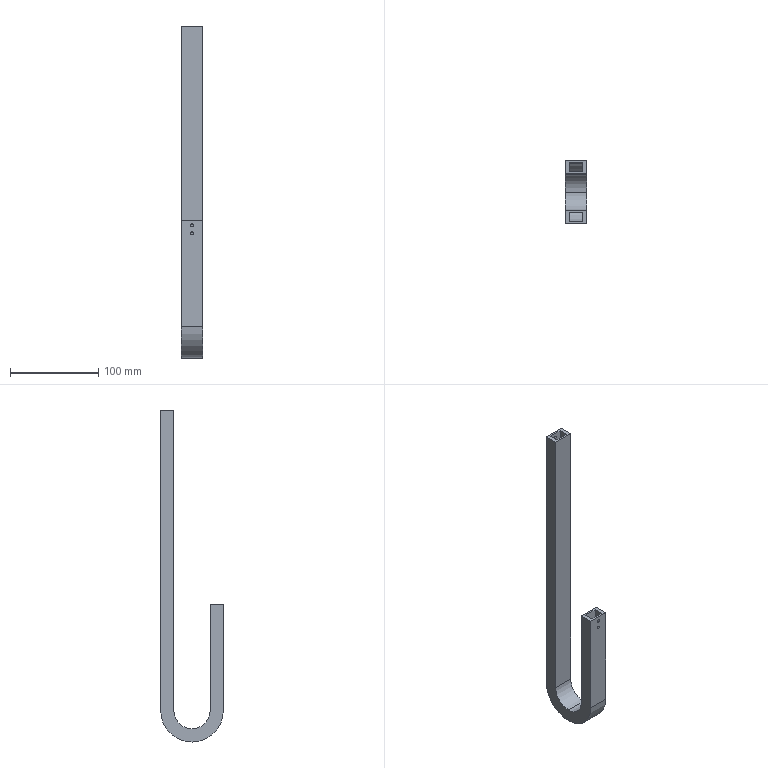Part | SolidWorks | features ICE 2, Sweep 1 | 1 solid | 30 faces | box 24 x 71 x 375.5 mm | volume 114976 mm3 | cylinder 16 | plane 14 | commonest cylinder face diameters 3.5 x8 41 x2 46 x2 66 x2 71 x2
STEP:
#1=CARTESIAN_POINT('',(-1.75,-5.,-14.5));
#2=VERTEX_POINT('',#1);
#3=CARTESIAN_POINT('',(1.75,-5.,-14.5));
#4=VERTEX_POINT('',#3);
#5=CARTESIAN_POINT('',(0.,-5.,-14.5));
#6=DIRECTION('',(0.,-1.,0.));
#7=DIRECTION('',(1.,0.,0.));
#8=AXIS2_PLACEMENT_3D('',#5,#6,#7);
#9=CIRCLE('',#8,1.75);
#10=EDGE_CURVE('',#2,#4,#9,.T.);
#11=ORIENTED_EDGE('',*,*,#10,.F.);
#12=CARTESIAN_POINT('',(-1.75,-7.5,-14.5));
#13=VERTEX_POINT('',#12);
#14=CARTESIAN_POINT('',(-1.75,-2.5,-14.5));
#15=DIRECTION('',(0.,-1.,0.));
#16=VECTOR('',#15,1000.);
#17=LINE('',#14,#16);
#18=EDGE_CURVE('',#2,#13,#17,.T.);
#19=ORIENTED_EDGE('',*,*,#18,.T.);
#20=CARTESIAN_POINT('',(1.75,-7.5,-14.5));
#21=VERTEX_POINT('',#20);
#22=CARTESIAN_POINT('',(0.,-7.5,-14.5));
#23=DIRECTION('',(0.,-1.,0.));
#24=DIRECTION('',(1.,0.,0.));
#25=AXIS2_PLACEMENT_3D('',#22,#23,#24);
#26=CIRCLE('',#25,1.75);
#27=EDGE_CURVE('',#13,#21,#26,.T.);
#28=ORIENTED_EDGE('',*,*,#27,.T.);
#29=CARTESIAN_POINT('',(1.75,-2.5,-14.5));
#30=DIRECTION('',(0.,-1.,0.));
#31=VECTOR('',#30,1000.);
#32=LINE('',#29,#31);
#33=EDGE_CURVE('',#4,#21,#32,.T.);
#34=ORIENTED_EDGE('',*,*,#33,.F.);
#35=EDGE_LOOP('',(#11,#19,#28,#34));
#36=FACE_OUTER_BOUND('',#35,.T.);
#37=CARTESIAN_POINT('',(0.,-2.5,-14.5));
#38=DIRECTION('',(0.,-1.,0.));
#39=DIRECTION('',(1.,0.,0.));
#40=AXIS2_PLACEMENT_3D('',#37,#38,#39);
#41=CYLINDRICAL_SURFACE('',#40,1.75);
#42=ADVANCED_FACE('',(#36),#41,.F.);
#43=CARTESIAN_POINT('',(-1.75,-5.,-5.5));
#44=VERTEX_POINT('',#43);
#45=CARTESIAN_POINT('',(1.75,-5.,-5.5));
#46=VERTEX_POINT('',#45);
#47=CARTESIAN_POINT('',(0.,-5.,-5.5));
#48=DIRECTION('',(0.,-1.,0.));
#49=DIRECTION('',(1.,0.,0.));
#50=AXIS2_PLACEMENT_3D('',#47,#48,#49);
#51=CIRCLE('',#50,1.75);
#52=EDGE_CURVE('',#44,#46,#51,.T.);
#53=ORIENTED_EDGE('',*,*,#52,.F.);
#54=CARTESIAN_POINT('',(-1.75,-7.5,-5.5));
#55=VERTEX_POINT('',#54);
#56=CARTESIAN_POINT('',(-1.75,-2.5,-5.5));
#57=DIRECTION('',(0.,-1.,0.));
#58=VECTOR('',#57,1000.);
#59=LINE('',#56,#58);
#60=EDGE_CURVE('',#44,#55,#59,.T.);
#61=ORIENTED_EDGE('',*,*,#60,.T.);
#62=CARTESIAN_POINT('',(1.75,-7.5,-5.5));
#63=VERTEX_POINT('',#62);
#64=CARTESIAN_POINT('',(0.,-7.5,-5.5));
#65=DIRECTION('',(0.,-1.,0.));
#66=DIRECTION('',(1.,0.,0.));
#67=AXIS2_PLACEMENT_3D('',#64,#65,#66);
#68=CIRCLE('',#67,1.75);
#69=EDGE_CURVE('',#55,#63,#68,.T.);
#70=ORIENTED_EDGE('',*,*,#69,.T.);
#71=CARTESIAN_POINT('',(1.75,-2.5,-5.5));
#72=DIRECTION('',(0.,-1.,0.));
#73=VECTOR('',#72,1000.);
#74=LINE('',#71,#73);
#75=EDGE_CURVE('',#46,#63,#74,.T.);
#76=ORIENTED_EDGE('',*,*,#75,.F.);
#77=EDGE_LOOP('',(#53,#61,#70,#76));
#78=FACE_OUTER_BOUND('',#77,.T.);
#79=CARTESIAN_POINT('',(0.,-2.5,-5.5));
#80=DIRECTION('',(0.,-1.,0.));
#81=DIRECTION('',(1.,0.,0.));
#82=AXIS2_PLACEMENT_3D('',#79,#80,#81);
#83=CYLINDRICAL_SURFACE('',#82,1.75);
#84=ADVANCED_FACE('',(#78),#83,.F.);
#85=CARTESIAN_POINT('',(-1.75,61.,205.5));
#86=VERTEX_POINT('',#85);
#87=CARTESIAN_POINT('',(1.75,61.,205.5));
#88=VERTEX_POINT('',#87);
#89=CARTESIAN_POINT('',(0.,61.,205.5));
#90=DIRECTION('',(0.,-1.,0.));
#91=DIRECTION('',(0.,0.,-1.));
#92=AXIS2_PLACEMENT_3D('',#89,#90,#91);
#93=CIRCLE('',#92,1.75);
#94=EDGE_CURVE('',#86,#88,#93,.T.);
#95=ORIENTED_EDGE('',*,*,#94,.T.);
#96=CARTESIAN_POINT('',(1.75,63.5,205.5));
#97=VERTEX_POINT('',#96);
#98=CARTESIAN_POINT('',(1.75,58.5,205.5));
#99=DIRECTION('',(0.,1.,0.));
#100=VECTOR('',#99,1000.);
#101=LINE('',#98,#100);
#102=EDGE_CURVE('',#88,#97,#101,.T.);
#103=ORIENTED_EDGE('',*,*,#102,.T.);
#104=CARTESIAN_POINT('',(-1.75,63.5,205.5));
#105=VERTEX_POINT('',#104);
#106=CARTESIAN_POINT('',(0.,63.5,205.5));
#107=DIRECTION('',(0.,1.,0.));
#108=DIRECTION('',(-1.,0.,0.));
#109=AXIS2_PLACEMENT_3D('',#106,#107,#108);
#110=CIRCLE('',#109,1.75);
#111=EDGE_CURVE('',#97,#105,#110,.T.);
#112=ORIENTED_EDGE('',*,*,#111,.T.);
#113=CARTESIAN_POINT('',(-1.75,58.5,205.5));
#114=DIRECTION('',(0.,1.,0.));
#115=VECTOR('',#114,1000.);
#116=LINE('',#113,#115);
#117=EDGE_CURVE('',#86,#105,#116,.T.);
#118=ORIENTED_EDGE('',*,*,#117,.F.);
#119=EDGE_LOOP('',(#95,#103,#112,#118));
#120=FACE_OUTER_BOUND('',#119,.T.);
#121=CARTESIAN_POINT('',(0.,58.5,205.5));
#122=DIRECTION('',(0.,1.,0.));
#123=DIRECTION('',(-1.,0.,0.));
#124=AXIS2_PLACEMENT_3D('',#121,#122,#123);
#125=CYLINDRICAL_SURFACE('',#124,1.75);
#126=ADVANCED_FACE('',(#120),#125,.F.);
#127=CARTESIAN_POINT('',(-1.75,61.,214.5));
#128=VERTEX_POINT('',#127);
#129=CARTESIAN_POINT('',(1.75,61.,214.5));
#130=VERTEX_POINT('',#129);
#131=CARTESIAN_POINT('',(0.,61.,214.5));
#132=DIRECTION('',(0.,-1.,0.));
#133=DIRECTION('',(0.,0.,-1.));
#134=AXIS2_PLACEMENT_3D('',#131,#132,#133);
#135=CIRCLE('',#134,1.75);
#136=EDGE_CURVE('',#128,#130,#135,.T.);
#137=ORIENTED_EDGE('',*,*,#136,.T.);
#138=CARTESIAN_POINT('',(1.75,63.5,214.5));
#139=VERTEX_POINT('',#138);
#140=CARTESIAN_POINT('',(1.75,58.5,214.5));
#141=DIRECTION('',(0.,1.,0.));
#142=VECTOR('',#141,1000.);
#143=LINE('',#140,#142);
#144=EDGE_CURVE('',#130,#139,#143,.T.);
#145=ORIENTED_EDGE('',*,*,#144,.T.);
#146=CARTESIAN_POINT('',(-1.75,63.5,214.5));
#147=VERTEX_POINT('',#146);
#148=CARTESIAN_POINT('',(0.,63.5,214.5));
#149=DIRECTION('',(0.,1.,0.));
#150=DIRECTION('',(-1.,0.,0.));
#151=AXIS2_PLACEMENT_3D('',#148,#149,#150);
#152=CIRCLE('',#151,1.75);
#153=EDGE_CURVE('',#139,#147,#152,.T.);
#154=ORIENTED_EDGE('',*,*,#153,.T.);
#155=CARTESIAN_POINT('',(-1.75,58.5,214.5));
#156=DIRECTION('',(0.,1.,0.));
#157=VECTOR('',#156,1000.);
#158=LINE('',#155,#157);
#159=EDGE_CURVE('',#128,#147,#158,.T.);
#160=ORIENTED_EDGE('',*,*,#159,.F.);
#161=EDGE_LOOP('',(#137,#145,#154,#160));
#162=FACE_OUTER_BOUND('',#161,.T.);
#163=CARTESIAN_POINT('',(0.,58.5,214.5));
#164=DIRECTION('',(0.,1.,0.));
#165=DIRECTION('',(-1.,0.,0.));
#166=AXIS2_PLACEMENT_3D('',#163,#164,#165);
#167=CYLINDRICAL_SURFACE('',#166,1.75);
#168=ADVANCED_FACE('',(#162),#167,.F.);
#169=CARTESIAN_POINT('',(-7.5,5.,-120.));
#170=VERTEX_POINT('',#169);
#171=CARTESIAN_POINT('',(-7.5,28.,-143.));
#172=VERTEX_POINT('',#171);
#173=CARTESIAN_POINT('',(-7.5,28.,-120.));
#174=DIRECTION('',(1.,0.,0.));
#175=DIRECTION('',(0.,0.,-1.));
#176=AXIS2_PLACEMENT_3D('',#173,#174,#175);
#177=CIRCLE('',#176,23.);
#178=EDGE_CURVE('',#170,#172,#177,.T.);
#179=ORIENTED_EDGE('',*,*,#178,.T.);
#180=CARTESIAN_POINT('',(7.5,28.,-143.));
#181=VERTEX_POINT('',#180);
#182=CARTESIAN_POINT('',(0.,28.,-143.));
#183=DIRECTION('',(1.,0.,0.));
#184=VECTOR('',#183,1000.);
#185=LINE('',#182,#184);
#186=EDGE_CURVE('',#172,#181,#185,.T.);
#187=ORIENTED_EDGE('',*,*,#186,.T.);
#188=CARTESIAN_POINT('',(7.5,5.,-120.));
#189=VERTEX_POINT('',#188);
#190=CARTESIAN_POINT('',(7.5,28.,-120.));
#191=DIRECTION('',(1.,0.,0.));
#192=DIRECTION('',(0.,0.,-1.));
#193=AXIS2_PLACEMENT_3D('',#190,#191,#192);
#194=CIRCLE('',#193,23.);
#195=EDGE_CURVE('',#189,#181,#194,.T.);
#196=ORIENTED_EDGE('',*,*,#195,.F.);
#197=CARTESIAN_POINT('',(7.5,5.,-120.));
#198=DIRECTION('',(-1.,0.,0.));
#199=VECTOR('',#198,1000.);
#200=LINE('',#197,#199);
#201=EDGE_CURVE('',#189,#170,#200,.T.);
#202=ORIENTED_EDGE('',*,*,#201,.T.);
#203=EDGE_LOOP('',(#179,#187,#196,#202));
#204=FACE_OUTER_BOUND('',#203,.T.);
#205=CARTESIAN_POINT('',(0.,28.,-120.));
#206=DIRECTION('',(1.,0.,0.));
#207=DIRECTION('',(0.,0.,-1.));
#208=AXIS2_PLACEMENT_3D('',#205,#206,#207);
#209=CYLINDRICAL_SURFACE('',#208,23.);
#210=ADVANCED_FACE('',(#204),#209,.T.);
#211=CARTESIAN_POINT('',(-7.5,28.,-153.));
#212=VERTEX_POINT('',#211);
#213=CARTESIAN_POINT('',(-7.5,61.,-120.));
#214=VERTEX_POINT('',#213);
#215=CARTESIAN_POINT('',(-7.5,28.,-120.));
#216=DIRECTION('',(1.,0.,0.));
#217=DIRECTION('',(0.,0.,-1.));
#218=AXIS2_PLACEMENT_3D('',#215,#216,#217);
#219=CIRCLE('',#218,33.);
#220=EDGE_CURVE('',#212,#214,#219,.T.);
#221=ORIENTED_EDGE('',*,*,#220,.F.);
#222=CARTESIAN_POINT('',(7.5,28.,-153.));
#223=VERTEX_POINT('',#222);
#224=CARTESIAN_POINT('',(0.,28.,-153.));
#225=DIRECTION('',(1.,0.,0.));
#226=VECTOR('',#225,1000.);
#227=LINE('',#224,#226);
#228=EDGE_CURVE('',#212,#223,#227,.T.);
#229=ORIENTED_EDGE('',*,*,#228,.T.);
#230=CARTESIAN_POINT('',(7.5,61.,-120.));
#231=VERTEX_POINT('',#230);
#232=CARTESIAN_POINT('',(7.5,28.,-120.));
#233=DIRECTION('',(1.,0.,0.));
#234=DIRECTION('',(0.,0.,-1.));
#235=AXIS2_PLACEMENT_3D('',#232,#233,#234);
#236=CIRCLE('',#235,33.);
#237=EDGE_CURVE('',#223,#231,#236,.T.);
#238=ORIENTED_EDGE('',*,*,#237,.T.);
#239=CARTESIAN_POINT('',(7.5,61.,-120.));
#240=DIRECTION('',(1.,0.,0.));
#241=VECTOR('',#240,1000.);
#242=LINE('',#239,#241);
#243=EDGE_CURVE('',#214,#231,#242,.T.);
#244=ORIENTED_EDGE('',*,*,#243,.F.);
#245=EDGE_LOOP('',(#221,#229,#238,#244));
#246=FACE_OUTER_BOUND('',#245,.T.);
#247=CARTESIAN_POINT('',(0.,28.,-120.));
#248=DIRECTION('',(1.,0.,0.));
#249=DIRECTION('',(0.,0.,-1.));
#250=AXIS2_PLACEMENT_3D('',#247,#248,#249);
#251=CYLINDRICAL_SURFACE('',#250,33.);
#252=ADVANCED_FACE('',(#246),#251,.F.);
#253=CARTESIAN_POINT('',(-12.,-7.5,-120.));
#254=VERTEX_POINT('',#253);
#255=CARTESIAN_POINT('',(-12.,28.,-155.5));
#256=VERTEX_POINT('',#255);
#257=CARTESIAN_POINT('',(-12.,28.,-120.));
#258=DIRECTION('',(1.,0.,0.));
#259=DIRECTION('',(0.,0.,-1.));
#260=AXIS2_PLACEMENT_3D('',#257,#258,#259);
#261=CIRCLE('',#260,35.5);
#262=EDGE_CURVE('',#254,#256,#261,.T.);
#263=ORIENTED_EDGE('',*,*,#262,.T.);
#264=CARTESIAN_POINT('',(12.,28.,-155.5));
#265=VERTEX_POINT('',#264);
#266=CARTESIAN_POINT('',(0.,28.,-155.5));
#267=DIRECTION('',(1.,0.,0.));
#268=VECTOR('',#267,1000.);
#269=LINE('',#266,#268);
#270=EDGE_CURVE('',#256,#265,#269,.T.);
#271=ORIENTED_EDGE('',*,*,#270,.T.);
#272=CARTESIAN_POINT('',(12.,-7.5,-120.));
#273=VERTEX_POINT('',#272);
#274=CARTESIAN_POINT('',(12.,28.,-120.));
#275=DIRECTION('',(1.,0.,0.));
#276=DIRECTION('',(0.,0.,-1.));
#277=AXIS2_PLACEMENT_3D('',#274,#275,#276);
#278=CIRCLE('',#277,35.5);
#279=EDGE_CURVE('',#273,#265,#278,.T.);
#280=ORIENTED_EDGE('',*,*,#279,.F.);
#281=CARTESIAN_POINT('',(12.,-7.5,-120.));
#282=DIRECTION('',(1.,0.,0.));
#283=VECTOR('',#282,1000.);
#284=LINE('',#281,#283);
#285=EDGE_CURVE('',#254,#273,#284,.T.);
#286=ORIENTED_EDGE('',*,*,#285,.F.);
#287=EDGE_LOOP('',(#263,#271,#280,#286));
#288=FACE_OUTER_BOUND('',#287,.T.);
#289=CARTESIAN_POINT('',(0.,28.,-120.));
#290=DIRECTION('',(1.,0.,0.));
#291=DIRECTION('',(0.,0.,-1.));
#292=AXIS2_PLACEMENT_3D('',#289,#290,#291);
#293=CYLINDRICAL_SURFACE('',#292,35.5);
#294=ADVANCED_FACE('',(#288),#293,.T.);
#295=CARTESIAN_POINT('',(-12.,28.,-140.5));
#296=VERTEX_POINT('',#295);
#297=CARTESIAN_POINT('',(-12.,48.5,-120.));
#298=VERTEX_POINT('',#297);
#299=CARTESIAN_POINT('',(-12.,28.,-120.));
#300=DIRECTION('',(1.,0.,0.));
#301=DIRECTION('',(0.,0.,-1.));
#302=AXIS2_PLACEMENT_3D('',#299,#300,#301);
#303=CIRCLE('',#302,20.5);
#304=EDGE_CURVE('',#296,#298,#303,.T.);
#305=ORIENTED_EDGE('',*,*,#304,.F.);
#306=CARTESIAN_POINT('',(12.,28.,-140.5));
#307=VERTEX_POINT('',#306);
#308=CARTESIAN_POINT('',(0.,28.,-140.5));
#309=DIRECTION('',(1.,0.,0.));
#310=VECTOR('',#309,1000.);
#311=LINE('',#308,#310);
#312=EDGE_CURVE('',#296,#307,#311,.T.);
#313=ORIENTED_EDGE('',*,*,#312,.T.);
#314=CARTESIAN_POINT('',(12.,48.5,-120.));
#315=VERTEX_POINT('',#314);
#316=CARTESIAN_POINT('',(12.,28.,-120.));
#317=DIRECTION('',(1.,0.,0.));
#318=DIRECTION('',(0.,0.,-1.));
#319=AXIS2_PLACEMENT_3D('',#316,#317,#318);
#320=CIRCLE('',#319,20.5);
#321=EDGE_CURVE('',#307,#315,#320,.T.);
#322=ORIENTED_EDGE('',*,*,#321,.T.);
#323=CARTESIAN_POINT('',(12.,48.5,-120.));
#324=DIRECTION('',(-1.,0.,0.));
#325=VECTOR('',#324,1000.);
#326=LINE('',#323,#325);
#327=EDGE_CURVE('',#315,#298,#326,.T.);
#328=ORIENTED_EDGE('',*,*,#327,.T.);
#329=EDGE_LOOP('',(#305,#313,#322,#328));
#330=FACE_OUTER_BOUND('',#329,.T.);
#331=CARTESIAN_POINT('',(0.,28.,-120.));
#332=DIRECTION('',(1.,0.,0.));
#333=DIRECTION('',(0.,0.,-1.));
#334=AXIS2_PLACEMENT_3D('',#331,#332,#333);
#335=CYLINDRICAL_SURFACE('',#334,20.5);
#336=ADVANCED_FACE('',(#330),#335,.F.);
#337=ORIENTED_EDGE('',*,*,#327,.F.);
#338=CARTESIAN_POINT('',(12.,48.5,220.));
#339=VERTEX_POINT('',#338);
#340=CARTESIAN_POINT('',(12.,48.5,-120.));
#341=DIRECTION('',(0.,0.,1.));
#342=VECTOR('',#341,1000.);
#343=LINE('',#340,#342);
#344=EDGE_CURVE('',#315,#339,#343,.T.);
#345=ORIENTED_EDGE('',*,*,#344,.T.);
#346=CARTESIAN_POINT('',(-12.,48.5,220.));
#347=VERTEX_POINT('',#346);
#348=CARTESIAN_POINT('',(12.,48.5,220.));
#349=DIRECTION('',(-1.,0.,0.));
#350=VECTOR('',#349,1000.);
#351=LINE('',#348,#350);
#352=EDGE_CURVE('',#339,#347,#351,.T.);
#353=ORIENTED_EDGE('',*,*,#352,.T.);
#354=CARTESIAN_POINT('',(-12.,48.5,-120.));
#355=DIRECTION('',(0.,0.,1.));
#356=VECTOR('',#355,1000.);
#357=LINE('',#354,#356);
#358=EDGE_CURVE('',#298,#347,#357,.T.);
#359=ORIENTED_EDGE('',*,*,#358,.F.);
#360=EDGE_LOOP('',(#337,#345,#353,#359));
#361=FACE_OUTER_BOUND('',#360,.T.);
#362=CARTESIAN_POINT('',(12.,48.5,-120.));
#363=DIRECTION('',(0.,1.,0.));
#364=DIRECTION('',(-1.,0.,0.));
#365=AXIS2_PLACEMENT_3D('',#362,#363,#364);
#366=PLANE('',#365);
#367=ADVANCED_FACE('',(#361),#366,.F.);
#368=CARTESIAN_POINT('',(0.,63.5,205.5));
#369=DIRECTION('',(0.,1.,0.));
#370=DIRECTION('',(-1.,0.,0.));
#371=AXIS2_PLACEMENT_3D('',#368,#369,#370);
#372=CIRCLE('',#371,1.75);
#373=EDGE_CURVE('',#105,#97,#372,.T.);
#374=ORIENTED_EDGE('',*,*,#373,.F.);
#375=ORIENTED_EDGE('',*,*,#111,.F.);
#376=EDGE_LOOP('',(#374,#375));
#377=FACE_BOUND('',#376,.T.);
#378=CARTESIAN_POINT('',(0.,63.5,214.5));
#379=DIRECTION('',(0.,1.,0.));
#380=DIRECTION('',(-1.,0.,0.));
#381=AXIS2_PLACEMENT_3D('',#378,#379,#380);
#382=CIRCLE('',#381,1.75);
#383=EDGE_CURVE('',#147,#139,#382,.T.);
#384=ORIENTED_EDGE('',*,*,#383,.F.);
#385=ORIENTED_EDGE('',*,*,#153,.F.);
#386=EDGE_LOOP('',(#384,#385));
#387=FACE_BOUND('',#386,.T.);
#388=CARTESIAN_POINT('',(-12.,63.5,-120.));
#389=VERTEX_POINT('',#388);
#390=CARTESIAN_POINT('',(12.,63.5,-120.));
#391=VERTEX_POINT('',#390);
#392=CARTESIAN_POINT('',(12.,63.5,-120.));
#393=DIRECTION('',(1.,0.,0.));
#394=VECTOR('',#393,1000.);
#395=LINE('',#392,#394);
#396=EDGE_CURVE('',#389,#391,#395,.T.);
#397=ORIENTED_EDGE('',*,*,#396,.F.);
#398=CARTESIAN_POINT('',(-12.,63.5,220.));
#399=VERTEX_POINT('',#398);
#400=CARTESIAN_POINT('',(-12.,63.5,-120.));
#401=DIRECTION('',(0.,0.,1.));
#402=VECTOR('',#401,1000.);
#403=LINE('',#400,#402);
#404=EDGE_CURVE('',#389,#399,#403,.T.);
#405=ORIENTED_EDGE('',*,*,#404,.T.);
#406=CARTESIAN_POINT('',(12.,63.5,220.));
#407=VERTEX_POINT('',#406);
#408=CARTESIAN_POINT('',(12.,63.5,220.));
#409=DIRECTION('',(1.,0.,0.));
#410=VECTOR('',#409,1000.);
#411=LINE('',#408,#410);
#412=EDGE_CURVE('',#399,#407,#411,.T.);
#413=ORIENTED_EDGE('',*,*,#412,.T.);
#414=CARTESIAN_POINT('',(12.,63.5,-120.));
#415=DIRECTION('',(0.,0.,1.));
#416=VECTOR('',#415,1000.);
#417=LINE('',#414,#416);
#418=EDGE_CURVE('',#391,#407,#417,.T.);
#419=ORIENTED_EDGE('',*,*,#418,.F.);
#420=EDGE_LOOP('',(#397,#405,#413,#419));
#421=FACE_OUTER_BOUND('',#420,.T.);
#422=CARTESIAN_POINT('',(12.,63.5,-120.));
#423=DIRECTION('',(0.,-1.,0.));
#424=DIRECTION('',(1.,0.,0.));
#425=AXIS2_PLACEMENT_3D('',#422,#423,#424);
#426=PLANE('',#425);
#427=ADVANCED_FACE('',(#377,#387,#421),#426,.F.);
#428=ORIENTED_EDGE('',*,*,#94,.F.);
#429=CARTESIAN_POINT('',(0.,61.,205.5));
#430=DIRECTION('',(0.,-1.,0.));
#431=DIRECTION('',(0.,0.,-1.));
#432=AXIS2_PLACEMENT_3D('',#429,#430,#431);
#433=CIRCLE('',#432,1.75);
#434=EDGE_CURVE('',#88,#86,#433,.T.);
#435=ORIENTED_EDGE('',*,*,#434,.F.);
#436=EDGE_LOOP('',(#428,#435));
#437=FACE_BOUND('',#436,.T.);
#438=ORIENTED_EDGE('',*,*,#136,.F.);
#439=CARTESIAN_POINT('',(0.,61.,214.5));
#440=DIRECTION('',(0.,-1.,0.));
#441=DIRECTION('',(0.,0.,-1.));
#442=AXIS2_PLACEMENT_3D('',#439,#440,#441);
#443=CIRCLE('',#442,1.75);
#444=EDGE_CURVE('',#130,#128,#443,.T.);
#445=ORIENTED_EDGE('',*,*,#444,.F.);
#446=EDGE_LOOP('',(#438,#445));
#447=FACE_BOUND('',#446,.T.);
#448=ORIENTED_EDGE('',*,*,#243,.T.);
#449=CARTESIAN_POINT('',(7.5,61.,220.));
#450=VERTEX_POINT('',#449);
#451=CARTESIAN_POINT('',(7.5,61.,-120.));
#452=DIRECTION('',(0.,0.,1.));
#453=VECTOR('',#452,1000.);
#454=LINE('',#451,#453);
#455=EDGE_CURVE('',#231,#450,#454,.T.);
#456=ORIENTED_EDGE('',*,*,#455,.T.);
#457=CARTESIAN_POINT('',(-7.5,61.,220.));
#458=VERTEX_POINT('',#457);
#459=CARTESIAN_POINT('',(7.5,61.,220.));
#460=DIRECTION('',(1.,0.,0.));
#461=VECTOR('',#460,1000.);
#462=LINE('',#459,#461);
#463=EDGE_CURVE('',#458,#450,#462,.T.);
#464=ORIENTED_EDGE('',*,*,#463,.F.);
#465=CARTESIAN_POINT('',(-7.5,61.,-120.));
#466=DIRECTION('',(0.,0.,1.));
#467=VECTOR('',#466,1000.);
#468=LINE('',#465,#467);
#469=EDGE_CURVE('',#214,#458,#468,.T.);
#470=ORIENTED_EDGE('',*,*,#469,.F.);
#471=EDGE_LOOP('',(#448,#456,#464,#470));
#472=FACE_OUTER_BOUND('',#471,.T.);
#473=CARTESIAN_POINT('',(7.5,61.,-120.));
#474=DIRECTION('',(0.,-1.,0.));
#475=DIRECTION('',(0.,0.,-1.));
#476=AXIS2_PLACEMENT_3D('',#473,#474,#475);
#477=PLANE('',#476);
#478=ADVANCED_FACE('',(#437,#447,#472),#477,.T.);
#479=CARTESIAN_POINT('',(7.5,51.,-120.));
#480=VERTEX_POINT('',#479);
#481=CARTESIAN_POINT('',(-7.5,51.,-120.));
#482=VERTEX_POINT('',#481);
#483=CARTESIAN_POINT('',(7.5,51.,-120.));
#484=DIRECTION('',(-1.,0.,0.));
#485=VECTOR('',#484,1000.);
#486=LINE('',#483,#485);
#487=EDGE_CURVE('',#480,#482,#486,.T.);
#488=ORIENTED_EDGE('',*,*,#487,.T.);
#489=CARTESIAN_POINT('',(-7.5,51.,220.));
#490=VERTEX_POINT('',#489);
#491=CARTESIAN_POINT('',(-7.5,51.,-120.));
#492=DIRECTION('',(0.,0.,1.));
#493=VECTOR('',#492,1000.);
#494=LINE('',#491,#493);
#495=EDGE_CURVE('',#482,#490,#494,.T.);
#496=ORIENTED_EDGE('',*,*,#495,.T.);
#497=CARTESIAN_POINT('',(7.5,51.,220.));
#498=VERTEX_POINT('',#497);
#499=CARTESIAN_POINT('',(7.5,51.,220.));
#500=DIRECTION('',(-1.,0.,0.));
#501=VECTOR('',#500,1000.);
#502=LINE('',#499,#501);
#503=EDGE_CURVE('',#498,#490,#502,.T.);
#504=ORIENTED_EDGE('',*,*,#503,.F.);
#505=CARTESIAN_POINT('',(7.5,51.,-120.));
#506=DIRECTION('',(0.,0.,1.));
#507=VECTOR('',#506,1000.);
#508=LINE('',#505,#507);
#509=EDGE_CURVE('',#480,#498,#508,.T.);
#510=ORIENTED_EDGE('',*,*,#509,.F.);
#511=EDGE_LOOP('',(#488,#496,#504,#510));
#512=FACE_OUTER_BOUND('',#511,.T.);
#513=CARTESIAN_POINT('',(7.5,51.,-120.));
#514=DIRECTION('',(0.,1.,0.));
#515=DIRECTION('',(0.,0.,1.));
#516=AXIS2_PLACEMENT_3D('',#513,#514,#515);
#517=PLANE('',#516);
#518=ADVANCED_FACE('',(#512),#517,.T.);
#519=ORIENTED_EDGE('',*,*,#312,.F.);
#520=CARTESIAN_POINT('',(-12.,7.5,-120.));
#521=VERTEX_POINT('',#520);
#522=CARTESIAN_POINT('',(-12.,28.,-120.));
#523=DIRECTION('',(1.,0.,0.));
#524=DIRECTION('',(0.,0.,-1.));
#525=AXIS2_PLACEMENT_3D('',#522,#523,#524);
#526=CIRCLE('',#525,20.5);
#527=EDGE_CURVE('',#521,#296,#526,.T.);
#528=ORIENTED_EDGE('',*,*,#527,.F.);
#529=CARTESIAN_POINT('',(12.,7.5,-120.));
#530=VERTEX_POINT('',#529);
#531=CARTESIAN_POINT('',(12.,7.5,-120.));
#532=DIRECTION('',(-1.,0.,0.));
#533=VECTOR('',#532,1000.);
#534=LINE('',#531,#533);
#535=EDGE_CURVE('',#530,#521,#534,.T.);
#536=ORIENTED_EDGE('',*,*,#535,.F.);
#537=CARTESIAN_POINT('',(12.,28.,-120.));
#538=DIRECTION('',(1.,0.,0.));
#539=DIRECTION('',(0.,0.,-1.));
#540=AXIS2_PLACEMENT_3D('',#537,#538,#539);
#541=CIRCLE('',#540,20.5);
#542=EDGE_CURVE('',#530,#307,#541,.T.);
#543=ORIENTED_EDGE('',*,*,#542,.T.);
#544=EDGE_LOOP('',(#519,#528,#536,#543));
#545=FACE_OUTER_BOUND('',#544,.T.);
#546=CARTESIAN_POINT('',(0.,28.,-120.));
#547=DIRECTION('',(1.,0.,0.));
#548=DIRECTION('',(0.,0.,-1.));
#549=AXIS2_PLACEMENT_3D('',#546,#547,#548);
#550=CYLINDRICAL_SURFACE('',#549,20.5);
#551=ADVANCED_FACE('',(#545),#550,.F.);
#552=ORIENTED_EDGE('',*,*,#270,.F.);
#553=CARTESIAN_POINT('',(-12.,28.,-120.));
#554=DIRECTION('',(1.,0.,0.));
#555=DIRECTION('',(0.,0.,-1.));
#556=AXIS2_PLACEMENT_3D('',#553,#554,#555);
#557=CIRCLE('',#556,35.5);
#558=EDGE_CURVE('',#256,#389,#557,.T.);
#559=ORIENTED_EDGE('',*,*,#558,.T.);
#560=ORIENTED_EDGE('',*,*,#396,.T.);
#561=CARTESIAN_POINT('',(12.,28.,-120.));
#562=DIRECTION('',(1.,0.,0.));
#563=DIRECTION('',(0.,0.,-1.));
#564=AXIS2_PLACEMENT_3D('',#561,#562,#563);
#565=CIRCLE('',#564,35.5);
#566=EDGE_CURVE('',#265,#391,#565,.T.);
#567=ORIENTED_EDGE('',*,*,#566,.F.);
#568=EDGE_LOOP('',(#552,#559,#560,#567));
#569=FACE_OUTER_BOUND('',#568,.T.);
#570=CARTESIAN_POINT('',(0.,28.,-120.));
#571=DIRECTION('',(1.,0.,0.));
#572=DIRECTION('',(0.,0.,-1.));
#573=AXIS2_PLACEMENT_3D('',#570,#571,#572);
#574=CYLINDRICAL_SURFACE('',#573,35.5);
#575=ADVANCED_FACE('',(#569),#574,.T.);
#576=ORIENTED_EDGE('',*,*,#228,.F.);
#577=CARTESIAN_POINT('',(-7.5,-5.,-120.));
#578=VERTEX_POINT('',#577);
#579=CARTESIAN_POINT('',(-7.5,28.,-120.));
#580=DIRECTION('',(1.,0.,0.));
#581=DIRECTION('',(0.,0.,-1.));
#582=AXIS2_PLACEMENT_3D('',#579,#580,#581);
#583=CIRCLE('',#582,33.);
#584=EDGE_CURVE('',#578,#212,#583,.T.);
#585=ORIENTED_EDGE('',*,*,#584,.F.);
#586=CARTESIAN_POINT('',(7.5,-5.,-120.));
#587=VERTEX_POINT('',#586);
#588=CARTESIAN_POINT('',(7.5,-5.,-120.));
#589=DIRECTION('',(1.,0.,0.));
#590=VECTOR('',#589,1000.);
#591=LINE('',#588,#590);
#592=EDGE_CURVE('',#578,#587,#591,.T.);
#593=ORIENTED_EDGE('',*,*,#592,.T.);
#594=CARTESIAN_POINT('',(7.5,28.,-120.));
#595=DIRECTION('',(1.,0.,0.));
#596=DIRECTION('',(0.,0.,-1.));
#597=AXIS2_PLACEMENT_3D('',#594,#595,#596);
#598=CIRCLE('',#597,33.);
#599=EDGE_CURVE('',#587,#223,#598,.T.);
#600=ORIENTED_EDGE('',*,*,#599,.T.);
#601=EDGE_LOOP('',(#576,#585,#593,#600));
#602=FACE_OUTER_BOUND('',#601,.T.);
#603=CARTESIAN_POINT('',(0.,28.,-120.));
#604=DIRECTION('',(1.,0.,0.));
#605=DIRECTION('',(0.,0.,-1.));
#606=AXIS2_PLACEMENT_3D('',#603,#604,#605);
#607=CYLINDRICAL_SURFACE('',#606,33.);
#608=ADVANCED_FACE('',(#602),#607,.F.);
#609=ORIENTED_EDGE('',*,*,#186,.F.);
#610=CARTESIAN_POINT('',(-7.5,28.,-120.));
#611=DIRECTION('',(1.,0.,0.));
#612=DIRECTION('',(0.,0.,-1.));
#613=AXIS2_PLACEMENT_3D('',#610,#611,#612);
#614=CIRCLE('',#613,23.);
#615=EDGE_CURVE('',#172,#482,#614,.T.);
#616=ORIENTED_EDGE('',*,*,#615,.T.);
#617=ORIENTED_EDGE('',*,*,#487,.F.);
#618=CARTESIAN_POINT('',(7.5,28.,-120.));
#619=DIRECTION('',(1.,0.,0.));
#620=DIRECTION('',(0.,0.,-1.));
#621=AXIS2_PLACEMENT_3D('',#618,#619,#620);
#622=CIRCLE('',#621,23.);
#623=EDGE_CURVE('',#181,#480,#622,.T.);
#624=ORIENTED_EDGE('',*,*,#623,.F.);
#625=EDGE_LOOP('',(#609,#616,#617,#624));
#626=FACE_OUTER_BOUND('',#625,.T.);
#627=CARTESIAN_POINT('',(0.,28.,-120.));
#628=DIRECTION('',(1.,0.,0.));
#629=DIRECTION('',(0.,0.,-1.));
#630=AXIS2_PLACEMENT_3D('',#627,#628,#629);
#631=CYLINDRICAL_SURFACE('',#630,23.);
#632=ADVANCED_FACE('',(#626),#631,.T.);
#633=CARTESIAN_POINT('',(-12.,7.5,0.));
#634=VERTEX_POINT('',#633);
#635=CARTESIAN_POINT('',(-12.,-7.5,0.));
#636=VERTEX_POINT('',#635);
#637=CARTESIAN_POINT('',(-12.,-7.5,0.));
#638=DIRECTION('',(0.,-1.,0.));
#639=VECTOR('',#638,1000.);
#640=LINE('',#637,#639);
#641=EDGE_CURVE('',#634,#636,#640,.T.);
#642=ORIENTED_EDGE('',*,*,#641,.F.);
#643=CARTESIAN_POINT('',(-12.,7.5,-120.));
#644=DIRECTION('',(0.,0.,1.));
#645=VECTOR('',#644,1000.);
#646=LINE('',#643,#645);
#647=EDGE_CURVE('',#521,#634,#646,.T.);
#648=ORIENTED_EDGE('',*,*,#647,.F.);
#649=ORIENTED_EDGE('',*,*,#527,.T.);
#650=ORIENTED_EDGE('',*,*,#304,.T.);
#651=ORIENTED_EDGE('',*,*,#358,.T.);
#652=CARTESIAN_POINT('',(-12.,63.5,220.));
#653=DIRECTION('',(0.,1.,0.));
#654=VECTOR('',#653,1000.);
#655=LINE('',#652,#654);
#656=EDGE_CURVE('',#347,#399,#655,.T.);
#657=ORIENTED_EDGE('',*,*,#656,.T.);
#658=ORIENTED_EDGE('',*,*,#404,.F.);
#659=ORIENTED_EDGE('',*,*,#558,.F.);
#660=ORIENTED_EDGE('',*,*,#262,.F.);
#661=CARTESIAN_POINT('',(-12.,-7.5,-120.));
#662=DIRECTION('',(0.,0.,1.));
#663=VECTOR('',#662,1000.);
#664=LINE('',#661,#663);
#665=EDGE_CURVE('',#254,#636,#664,.T.);
#666=ORIENTED_EDGE('',*,*,#665,.T.);
#667=EDGE_LOOP('',(#642,#648,#649,#650,#651,#657,#658,#659,#660,#666));
#668=FACE_OUTER_BOUND('',#667,.T.);
#669=CARTESIAN_POINT('',(-12.,-7.5,-120.));
#670=DIRECTION('',(-1.,0.,0.));
#671=DIRECTION('',(0.,0.,1.));
#672=AXIS2_PLACEMENT_3D('',#669,#670,#671);
#673=PLANE('',#672);
#674=ADVANCED_FACE('',(#668),#673,.T.);
#675=CARTESIAN_POINT('',(12.,7.5,0.));
#676=VERTEX_POINT('',#675);
#677=CARTESIAN_POINT('',(12.,7.5,0.));
#678=DIRECTION('',(-1.,0.,0.));
#679=VECTOR('',#678,1000.);
#680=LINE('',#677,#679);
#681=EDGE_CURVE('',#676,#634,#680,.T.);
#682=ORIENTED_EDGE('',*,*,#681,.F.);
#683=CARTESIAN_POINT('',(12.,7.5,-120.));
#684=DIRECTION('',(0.,0.,1.));
#685=VECTOR('',#684,1000.);
#686=LINE('',#683,#685);
#687=EDGE_CURVE('',#530,#676,#686,.T.);
#688=ORIENTED_EDGE('',*,*,#687,.F.);
#689=ORIENTED_EDGE('',*,*,#535,.T.);
#690=ORIENTED_EDGE('',*,*,#647,.T.);
#691=EDGE_LOOP('',(#682,#688,#689,#690));
#692=FACE_OUTER_BOUND('',#691,.T.);
#693=CARTESIAN_POINT('',(12.,7.5,-120.));
#694=DIRECTION('',(0.,1.,0.));
#695=DIRECTION('',(-1.,0.,0.));
#696=AXIS2_PLACEMENT_3D('',#693,#694,#695);
#697=PLANE('',#696);
#698=ADVANCED_FACE('',(#692),#697,.T.);
#699=CARTESIAN_POINT('',(12.,-7.5,0.));
#700=VERTEX_POINT('',#699);
#701=CARTESIAN_POINT('',(12.,-7.5,0.));
#702=DIRECTION('',(0.,1.,0.));
#703=VECTOR('',#702,1000.);
#704=LINE('',#701,#703);
#705=EDGE_CURVE('',#700,#676,#704,.T.);
#706=ORIENTED_EDGE('',*,*,#705,.F.);
#707=CARTESIAN_POINT('',(12.,-7.5,-120.));
#708=DIRECTION('',(0.,0.,1.));
#709=VECTOR('',#708,1000.);
#710=LINE('',#707,#709);
#711=EDGE_CURVE('',#273,#700,#710,.T.);
#712=ORIENTED_EDGE('',*,*,#711,.F.);
#713=ORIENTED_EDGE('',*,*,#279,.T.);
#714=ORIENTED_EDGE('',*,*,#566,.T.);
#715=ORIENTED_EDGE('',*,*,#418,.T.);
#716=CARTESIAN_POINT('',(12.,63.5,220.));
#717=DIRECTION('',(0.,-1.,0.));
#718=VECTOR('',#717,1000.);
#719=LINE('',#716,#718);
#720=EDGE_CURVE('',#407,#339,#719,.T.);
#721=ORIENTED_EDGE('',*,*,#720,.T.);
#722=ORIENTED_EDGE('',*,*,#344,.F.);
#723=ORIENTED_EDGE('',*,*,#321,.F.);
#724=ORIENTED_EDGE('',*,*,#542,.F.);
#725=ORIENTED_EDGE('',*,*,#687,.T.);
#726=EDGE_LOOP('',(#706,#712,#713,#714,#715,#721,#722,#723,#724,#725));
#727=FACE_OUTER_BOUND('',#726,.T.);
#728=CARTESIAN_POINT('',(12.,-7.5,-120.));
#729=DIRECTION('',(1.,0.,0.));
#730=DIRECTION('',(0.,0.,-1.));
#731=AXIS2_PLACEMENT_3D('',#728,#729,#730);
#732=PLANE('',#731);
#733=ADVANCED_FACE('',(#727),#732,.T.);
#734=CARTESIAN_POINT('',(-7.5,5.,0.));
#735=VERTEX_POINT('',#734);
#736=CARTESIAN_POINT('',(-7.5,-5.,0.));
#737=VERTEX_POINT('',#736);
#738=CARTESIAN_POINT('',(-7.5,-5.,0.));
#739=DIRECTION('',(0.,-1.,0.));
#740=VECTOR('',#739,1000.);
#741=LINE('',#738,#740);
#742=EDGE_CURVE('',#735,#737,#741,.T.);
#743=ORIENTED_EDGE('',*,*,#742,.T.);
#744=CARTESIAN_POINT('',(-7.5,-5.,-120.));
#745=DIRECTION('',(0.,0.,1.));
#746=VECTOR('',#745,1000.);
#747=LINE('',#744,#746);
#748=EDGE_CURVE('',#578,#737,#747,.T.);
#749=ORIENTED_EDGE('',*,*,#748,.F.);
#750=ORIENTED_EDGE('',*,*,#584,.T.);
#751=ORIENTED_EDGE('',*,*,#220,.T.);
#752=ORIENTED_EDGE('',*,*,#469,.T.);
#753=CARTESIAN_POINT('',(-7.5,61.,220.));
#754=DIRECTION('',(0.,1.,0.));
#755=VECTOR('',#754,1000.);
#756=LINE('',#753,#755);
#757=EDGE_CURVE('',#490,#458,#756,.T.);
#758=ORIENTED_EDGE('',*,*,#757,.F.);
#759=ORIENTED_EDGE('',*,*,#495,.F.);
#760=ORIENTED_EDGE('',*,*,#615,.F.);
#761=ORIENTED_EDGE('',*,*,#178,.F.);
#762=CARTESIAN_POINT('',(-7.5,5.,-120.));
#763=DIRECTION('',(0.,0.,1.));
#764=VECTOR('',#763,1000.);
#765=LINE('',#762,#764);
#766=EDGE_CURVE('',#170,#735,#765,.T.);
#767=ORIENTED_EDGE('',*,*,#766,.T.);
#768=EDGE_LOOP('',(#743,#749,#750,#751,#752,#758,#759,#760,#761,#767));
#769=FACE_OUTER_BOUND('',#768,.T.);
#770=CARTESIAN_POINT('',(-7.5,-5.,-120.));
#771=DIRECTION('',(-1.,0.,0.));
#772=DIRECTION('',(0.,0.,1.));
#773=AXIS2_PLACEMENT_3D('',#770,#771,#772);
#774=PLANE('',#773);
#775=ADVANCED_FACE('',(#769),#774,.F.);
#776=CARTESIAN_POINT('',(0.,-5.,-14.5));
#777=DIRECTION('',(0.,-1.,0.));
#778=DIRECTION('',(1.,0.,0.));
#779=AXIS2_PLACEMENT_3D('',#776,#777,#778);
#780=CIRCLE('',#779,1.75);
#781=EDGE_CURVE('',#4,#2,#780,.T.);
#782=ORIENTED_EDGE('',*,*,#781,.T.);
#783=ORIENTED_EDGE('',*,*,#10,.T.);
#784=EDGE_LOOP('',(#782,#783));
#785=FACE_BOUND('',#784,.T.);
#786=CARTESIAN_POINT('',(0.,-5.,-5.5));
#787=DIRECTION('',(0.,-1.,0.));
#788=DIRECTION('',(1.,0.,0.));
#789=AXIS2_PLACEMENT_3D('',#786,#787,#788);
#790=CIRCLE('',#789,1.75);
#791=EDGE_CURVE('',#46,#44,#790,.T.);
#792=ORIENTED_EDGE('',*,*,#791,.T.);
#793=ORIENTED_EDGE('',*,*,#52,.T.);
#794=EDGE_LOOP('',(#792,#793));
#795=FACE_BOUND('',#794,.T.);
#796=CARTESIAN_POINT('',(7.5,-5.,0.));
#797=VERTEX_POINT('',#796);
#798=CARTESIAN_POINT('',(7.5,-5.,0.));
#799=DIRECTION('',(1.,0.,0.));
#800=VECTOR('',#799,1000.);
#801=LINE('',#798,#800);
#802=EDGE_CURVE('',#737,#797,#801,.T.);
#803=ORIENTED_EDGE('',*,*,#802,.T.);
#804=CARTESIAN_POINT('',(7.5,-5.,-120.));
#805=DIRECTION('',(0.,0.,1.));
#806=VECTOR('',#805,1000.);
#807=LINE('',#804,#806);
#808=EDGE_CURVE('',#587,#797,#807,.T.);
#809=ORIENTED_EDGE('',*,*,#808,.F.);
#810=ORIENTED_EDGE('',*,*,#592,.F.);
#811=ORIENTED_EDGE('',*,*,#748,.T.);
#812=EDGE_LOOP('',(#803,#809,#810,#811));
#813=FACE_OUTER_BOUND('',#812,.T.);
#814=CARTESIAN_POINT('',(7.5,-5.,-120.));
#815=DIRECTION('',(0.,-1.,0.));
#816=DIRECTION('',(1.,0.,0.));
#817=AXIS2_PLACEMENT_3D('',#814,#815,#816);
#818=PLANE('',#817);
#819=ADVANCED_FACE('',(#785,#795,#813),#818,.F.);
#820=CARTESIAN_POINT('',(7.5,5.,0.));
#821=VERTEX_POINT('',#820);
#822=CARTESIAN_POINT('',(7.5,-5.,0.));
#823=DIRECTION('',(0.,1.,0.));
#824=VECTOR('',#823,1000.);
#825=LINE('',#822,#824);
#826=EDGE_CURVE('',#797,#821,#825,.T.);
#827=ORIENTED_EDGE('',*,*,#826,.T.);
#828=CARTESIAN_POINT('',(7.5,5.,-120.));
#829=DIRECTION('',(0.,0.,1.));
#830=VECTOR('',#829,1000.);
#831=LINE('',#828,#830);
#832=EDGE_CURVE('',#189,#821,#831,.T.);
#833=ORIENTED_EDGE('',*,*,#832,.F.);
#834=ORIENTED_EDGE('',*,*,#195,.T.);
#835=ORIENTED_EDGE('',*,*,#623,.T.);
#836=ORIENTED_EDGE('',*,*,#509,.T.);
#837=CARTESIAN_POINT('',(7.5,61.,220.));
#838=DIRECTION('',(0.,-1.,0.));
#839=VECTOR('',#838,1000.);
#840=LINE('',#837,#839);
#841=EDGE_CURVE('',#450,#498,#840,.T.);
#842=ORIENTED_EDGE('',*,*,#841,.F.);
#843=ORIENTED_EDGE('',*,*,#455,.F.);
#844=ORIENTED_EDGE('',*,*,#237,.F.);
#845=ORIENTED_EDGE('',*,*,#599,.F.);
#846=ORIENTED_EDGE('',*,*,#808,.T.);
#847=EDGE_LOOP('',(#827,#833,#834,#835,#836,#842,#843,#844,#845,#846));
#848=FACE_OUTER_BOUND('',#847,.T.);
#849=CARTESIAN_POINT('',(7.5,-5.,-120.));
#850=DIRECTION('',(1.,0.,0.));
#851=DIRECTION('',(0.,0.,-1.));
#852=AXIS2_PLACEMENT_3D('',#849,#850,#851);
#853=PLANE('',#852);
#854=ADVANCED_FACE('',(#848),#853,.F.);
#855=CARTESIAN_POINT('',(7.5,5.,0.));
#856=DIRECTION('',(-1.,0.,0.));
#857=VECTOR('',#856,1000.);
#858=LINE('',#855,#857);
#859=EDGE_CURVE('',#821,#735,#858,.T.);
#860=ORIENTED_EDGE('',*,*,#859,.T.);
#861=ORIENTED_EDGE('',*,*,#766,.F.);
#862=ORIENTED_EDGE('',*,*,#201,.F.);
#863=ORIENTED_EDGE('',*,*,#832,.T.);
#864=EDGE_LOOP('',(#860,#861,#862,#863));
#865=FACE_OUTER_BOUND('',#864,.T.);
#866=CARTESIAN_POINT('',(7.5,5.,-120.));
#867=DIRECTION('',(0.,1.,0.));
#868=DIRECTION('',(-1.,0.,0.));
#869=AXIS2_PLACEMENT_3D('',#866,#867,#868);
#870=PLANE('',#869);
#871=ADVANCED_FACE('',(#865),#870,.F.);
#872=CARTESIAN_POINT('',(0.,-7.5,-14.5));
#873=DIRECTION('',(0.,-1.,0.));
#874=DIRECTION('',(1.,0.,0.));
#875=AXIS2_PLACEMENT_3D('',#872,#873,#874);
#876=CIRCLE('',#875,1.75);
#877=EDGE_CURVE('',#21,#13,#876,.T.);
#878=ORIENTED_EDGE('',*,*,#877,.F.);
#879=ORIENTED_EDGE('',*,*,#27,.F.);
#880=EDGE_LOOP('',(#878,#879));
#881=FACE_BOUND('',#880,.T.);
#882=CARTESIAN_POINT('',(0.,-7.5,-5.5));
#883=DIRECTION('',(0.,-1.,0.));
#884=DIRECTION('',(1.,0.,0.));
#885=AXIS2_PLACEMENT_3D('',#882,#883,#884);
#886=CIRCLE('',#885,1.75);
#887=EDGE_CURVE('',#63,#55,#886,.T.);
#888=ORIENTED_EDGE('',*,*,#887,.F.);
#889=ORIENTED_EDGE('',*,*,#69,.F.);
#890=EDGE_LOOP('',(#888,#889));
#891=FACE_BOUND('',#890,.T.);
#892=CARTESIAN_POINT('',(12.,-7.5,0.));
#893=DIRECTION('',(1.,0.,0.));
#894=VECTOR('',#893,1000.);
#895=LINE('',#892,#894);
#896=EDGE_CURVE('',#636,#700,#895,.T.);
#897=ORIENTED_EDGE('',*,*,#896,.F.);
#898=ORIENTED_EDGE('',*,*,#665,.F.);
#899=ORIENTED_EDGE('',*,*,#285,.T.);
#900=ORIENTED_EDGE('',*,*,#711,.T.);
#901=EDGE_LOOP('',(#897,#898,#899,#900));
#902=FACE_OUTER_BOUND('',#901,.T.);
#903=CARTESIAN_POINT('',(12.,-7.5,-120.));
#904=DIRECTION('',(0.,-1.,0.));
#905=DIRECTION('',(1.,0.,0.));
#906=AXIS2_PLACEMENT_3D('',#903,#904,#905);
#907=PLANE('',#906);
#908=ADVANCED_FACE('',(#881,#891,#902),#907,.T.);
#909=ORIENTED_EDGE('',*,*,#757,.T.);
#910=ORIENTED_EDGE('',*,*,#463,.T.);
#911=ORIENTED_EDGE('',*,*,#841,.T.);
#912=ORIENTED_EDGE('',*,*,#503,.T.);
#913=EDGE_LOOP('',(#909,#910,#911,#912));
#914=FACE_BOUND('',#913,.T.);
#915=ORIENTED_EDGE('',*,*,#656,.F.);
#916=ORIENTED_EDGE('',*,*,#352,.F.);
#917=ORIENTED_EDGE('',*,*,#720,.F.);
#918=ORIENTED_EDGE('',*,*,#412,.F.);
#919=EDGE_LOOP('',(#915,#916,#917,#918));
#920=FACE_OUTER_BOUND('',#919,.T.);
#921=CARTESIAN_POINT('',(0.,56.,220.));
#922=DIRECTION('',(0.,0.,-1.));
#923=DIRECTION('',(1.,0.,0.));
#924=AXIS2_PLACEMENT_3D('',#921,#922,#923);
#925=PLANE('',#924);
#926=ADVANCED_FACE('',(#914,#920),#925,.F.);
#927=ORIENTED_EDGE('',*,*,#742,.F.);
#928=ORIENTED_EDGE('',*,*,#859,.F.);
#929=ORIENTED_EDGE('',*,*,#826,.F.);
#930=ORIENTED_EDGE('',*,*,#802,.F.);
#931=EDGE_LOOP('',(#927,#928,#929,#930));
#932=FACE_BOUND('',#931,.T.);
#933=ORIENTED_EDGE('',*,*,#641,.T.);
#934=ORIENTED_EDGE('',*,*,#896,.T.);
#935=ORIENTED_EDGE('',*,*,#705,.T.);
#936=ORIENTED_EDGE('',*,*,#681,.T.);
#937=EDGE_LOOP('',(#933,#934,#935,#936));
#938=FACE_OUTER_BOUND('',#937,.T.);
#939=CARTESIAN_POINT('',(0.,0.,0.));
#940=DIRECTION('',(0.,0.,1.));
#941=DIRECTION('',(1.,0.,0.));
#942=AXIS2_PLACEMENT_3D('',#939,#940,#941);
#943=PLANE('',#942);
#944=ADVANCED_FACE('',(#932,#938),#943,.T.);
#945=ORIENTED_EDGE('',*,*,#144,.F.);
#946=ORIENTED_EDGE('',*,*,#444,.T.);
#947=ORIENTED_EDGE('',*,*,#159,.T.);
#948=ORIENTED_EDGE('',*,*,#383,.T.);
#949=EDGE_LOOP('',(#945,#946,#947,#948));
#950=FACE_OUTER_BOUND('',#949,.T.);
#951=CARTESIAN_POINT('',(0.,58.5,214.5));
#952=DIRECTION('',(0.,1.,0.));
#953=DIRECTION('',(-1.,0.,0.));
#954=AXIS2_PLACEMENT_3D('',#951,#952,#953);
#955=CYLINDRICAL_SURFACE('',#954,1.75);
#956=ADVANCED_FACE('',(#950),#955,.F.);
#957=ORIENTED_EDGE('',*,*,#102,.F.);
#958=ORIENTED_EDGE('',*,*,#434,.T.);
#959=ORIENTED_EDGE('',*,*,#117,.T.);
#960=ORIENTED_EDGE('',*,*,#373,.T.);
#961=EDGE_LOOP('',(#957,#958,#959,#960));
#962=FACE_OUTER_BOUND('',#961,.T.);
#963=CARTESIAN_POINT('',(0.,58.5,205.5));
#964=DIRECTION('',(0.,1.,0.));
#965=DIRECTION('',(-1.,0.,0.));
#966=AXIS2_PLACEMENT_3D('',#963,#964,#965);
#967=CYLINDRICAL_SURFACE('',#966,1.75);
#968=ADVANCED_FACE('',(#962),#967,.F.);
#969=ORIENTED_EDGE('',*,*,#60,.F.);
#970=ORIENTED_EDGE('',*,*,#791,.F.);
#971=ORIENTED_EDGE('',*,*,#75,.T.);
#972=ORIENTED_EDGE('',*,*,#887,.T.);
#973=EDGE_LOOP('',(#969,#970,#971,#972));
#974=FACE_OUTER_BOUND('',#973,.T.);
#975=CARTESIAN_POINT('',(0.,-2.5,-5.5));
#976=DIRECTION('',(0.,-1.,0.));
#977=DIRECTION('',(1.,0.,0.));
#978=AXIS2_PLACEMENT_3D('',#975,#976,#977);
#979=CYLINDRICAL_SURFACE('',#978,1.75);
#980=ADVANCED_FACE('',(#974),#979,.F.);
#981=ORIENTED_EDGE('',*,*,#18,.F.);
#982=ORIENTED_EDGE('',*,*,#781,.F.);
#983=ORIENTED_EDGE('',*,*,#33,.T.);
#984=ORIENTED_EDGE('',*,*,#877,.T.);
#985=EDGE_LOOP('',(#981,#982,#983,#984));
#986=FACE_OUTER_BOUND('',#985,.T.);
#987=CARTESIAN_POINT('',(0.,-2.5,-14.5));
#988=DIRECTION('',(0.,-1.,0.));
#989=DIRECTION('',(1.,0.,0.));
#990=AXIS2_PLACEMENT_3D('',#987,#988,#989);
#991=CYLINDRICAL_SURFACE('',#990,1.75);
#992=ADVANCED_FACE('',(#986),#991,.F.);
#993=CLOSED_SHELL('',(#42,#84,#126,#168,#210,#252,#294,#336,#367,#427,#478,#518,#551,#575,#608,#632,#674,#698,#733,#775,#819,#854,#871,#908,#926,#944,#956,#968,#980,#992));
#994=MANIFOLD_SOLID_BREP('',#993);
#995=CARTESIAN_POINT('',(0.,0.,0.));
#996=DIRECTION('',(0.,0.,1.));
#997=DIRECTION('',(1.,0.,0.));
#998=AXIS2_PLACEMENT_3D('',#995,#996,#997);
#999=(LENGTH_UNIT()NAMED_UNIT(*)SI_UNIT(.MILLI.,.METRE.));
#1000=UNCERTAINTY_MEASURE_WITH_UNIT(LENGTH_MEASURE(0.00001),#999,'','');
#1001=(NAMED_UNIT(*)PLANE_ANGLE_UNIT()SI_UNIT($,.RADIAN.));
#1002=(NAMED_UNIT(*)SI_UNIT($,.STERADIAN.)SOLID_ANGLE_UNIT());
#1003=(GEOMETRIC_REPRESENTATION_CONTEXT(3)GLOBAL_UNCERTAINTY_ASSIGNED_CONTEXT((#1000))GLOBAL_UNIT_ASSIGNED_CONTEXT((#999,#1001,#1002))REPRESENTATION_CONTEXT('',''));
#1004=ADVANCED_BREP_SHAPE_REPRESENTATION('',(#994,#998),#1003);